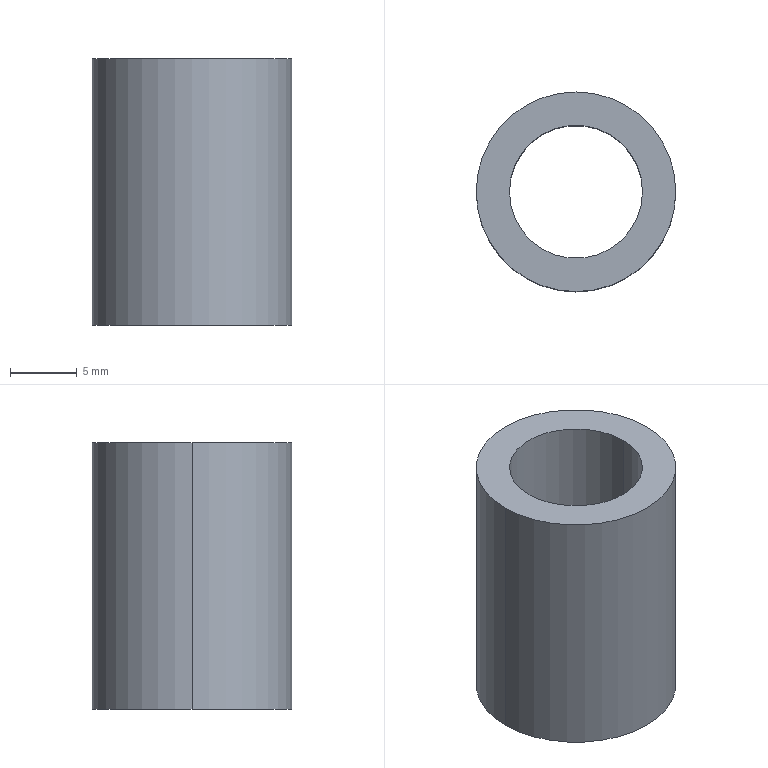Part | SolidWorks | features Extrusion 1 | 1 solid | 6 faces | box 15 x 15 x 20 mm | volume 1963 mm3 | cylinder 4 | plane 2 | commonest cylinder face diameters 10 x2 15 x2
STEP:
#1=CARTESIAN_POINT('',(-5.,0.,10.));
#2=VERTEX_POINT('',#1);
#3=CARTESIAN_POINT('',(5.,0.,10.));
#4=VERTEX_POINT('',#3);
#5=CARTESIAN_POINT('',(0.,0.,10.));
#6=DIRECTION('',(0.,0.,1.));
#7=DIRECTION('',(1.,0.,0.));
#8=AXIS2_PLACEMENT_3D('',#5,#6,#7);
#9=CIRCLE('',#8,5.);
#10=EDGE_CURVE('',#2,#4,#9,.T.);
#11=ORIENTED_EDGE('',*,*,#10,.T.);
#12=CARTESIAN_POINT('',(5.,0.,-10.));
#13=VERTEX_POINT('',#12);
#14=CARTESIAN_POINT('',(5.,0.,10.));
#15=DIRECTION('',(0.,0.,-1.));
#16=VECTOR('',#15,1000.);
#17=LINE('',#14,#16);
#18=EDGE_CURVE('',#4,#13,#17,.T.);
#19=ORIENTED_EDGE('',*,*,#18,.T.);
#20=CARTESIAN_POINT('',(-5.,0.,-10.));
#21=VERTEX_POINT('',#20);
#22=CARTESIAN_POINT('',(0.,0.,-10.));
#23=DIRECTION('',(0.,0.,1.));
#24=DIRECTION('',(1.,0.,0.));
#25=AXIS2_PLACEMENT_3D('',#22,#23,#24);
#26=CIRCLE('',#25,5.);
#27=EDGE_CURVE('',#21,#13,#26,.T.);
#28=ORIENTED_EDGE('',*,*,#27,.F.);
#29=CARTESIAN_POINT('',(-5.,0.,10.));
#30=DIRECTION('',(0.,0.,-1.));
#31=VECTOR('',#30,1000.);
#32=LINE('',#29,#31);
#33=EDGE_CURVE('',#2,#21,#32,.T.);
#34=ORIENTED_EDGE('',*,*,#33,.F.);
#35=EDGE_LOOP('',(#11,#19,#28,#34));
#36=FACE_OUTER_BOUND('',#35,.T.);
#37=CARTESIAN_POINT('',(0.,0.,10.));
#38=DIRECTION('',(0.,0.,-1.));
#39=DIRECTION('',(-1.,0.,0.));
#40=AXIS2_PLACEMENT_3D('',#37,#38,#39);
#41=CYLINDRICAL_SURFACE('',#40,5.);
#42=ADVANCED_FACE('',(#36),#41,.F.);
#43=CARTESIAN_POINT('',(7.5,0.,10.));
#44=VERTEX_POINT('',#43);
#45=CARTESIAN_POINT('',(-7.5,0.,10.));
#46=VERTEX_POINT('',#45);
#47=CARTESIAN_POINT('',(0.,0.,10.));
#48=DIRECTION('',(0.,0.,1.));
#49=DIRECTION('',(1.,0.,0.));
#50=AXIS2_PLACEMENT_3D('',#47,#48,#49);
#51=CIRCLE('',#50,7.5);
#52=EDGE_CURVE('',#44,#46,#51,.T.);
#53=ORIENTED_EDGE('',*,*,#52,.F.);
#54=CARTESIAN_POINT('',(7.5,0.,-10.));
#55=VERTEX_POINT('',#54);
#56=CARTESIAN_POINT('',(7.5,0.,10.));
#57=DIRECTION('',(0.,0.,-1.));
#58=VECTOR('',#57,1000.);
#59=LINE('',#56,#58);
#60=EDGE_CURVE('',#44,#55,#59,.T.);
#61=ORIENTED_EDGE('',*,*,#60,.T.);
#62=CARTESIAN_POINT('',(-7.5,0.,-10.));
#63=VERTEX_POINT('',#62);
#64=CARTESIAN_POINT('',(0.,0.,-10.));
#65=DIRECTION('',(0.,0.,1.));
#66=DIRECTION('',(1.,0.,0.));
#67=AXIS2_PLACEMENT_3D('',#64,#65,#66);
#68=CIRCLE('',#67,7.5);
#69=EDGE_CURVE('',#55,#63,#68,.T.);
#70=ORIENTED_EDGE('',*,*,#69,.T.);
#71=CARTESIAN_POINT('',(-7.5,0.,10.));
#72=DIRECTION('',(0.,0.,-1.));
#73=VECTOR('',#72,1000.);
#74=LINE('',#71,#73);
#75=EDGE_CURVE('',#46,#63,#74,.T.);
#76=ORIENTED_EDGE('',*,*,#75,.F.);
#77=EDGE_LOOP('',(#53,#61,#70,#76));
#78=FACE_OUTER_BOUND('',#77,.T.);
#79=CARTESIAN_POINT('',(0.,0.,10.));
#80=DIRECTION('',(0.,0.,-1.));
#81=DIRECTION('',(-1.,0.,0.));
#82=AXIS2_PLACEMENT_3D('',#79,#80,#81);
#83=CYLINDRICAL_SURFACE('',#82,7.5);
#84=ADVANCED_FACE('',(#78),#83,.T.);
#85=CARTESIAN_POINT('',(0.,0.,10.));
#86=DIRECTION('',(0.,0.,1.));
#87=DIRECTION('',(1.,0.,0.));
#88=AXIS2_PLACEMENT_3D('',#85,#86,#87);
#89=CIRCLE('',#88,7.5);
#90=EDGE_CURVE('',#46,#44,#89,.T.);
#91=ORIENTED_EDGE('',*,*,#90,.T.);
#92=ORIENTED_EDGE('',*,*,#52,.T.);
#93=EDGE_LOOP('',(#91,#92));
#94=FACE_OUTER_BOUND('',#93,.T.);
#95=ORIENTED_EDGE('',*,*,#10,.F.);
#96=CARTESIAN_POINT('',(0.,0.,10.));
#97=DIRECTION('',(0.,0.,1.));
#98=DIRECTION('',(1.,0.,0.));
#99=AXIS2_PLACEMENT_3D('',#96,#97,#98);
#100=CIRCLE('',#99,5.);
#101=EDGE_CURVE('',#4,#2,#100,.T.);
#102=ORIENTED_EDGE('',*,*,#101,.F.);
#103=EDGE_LOOP('',(#95,#102));
#104=FACE_BOUND('',#103,.T.);
#105=CARTESIAN_POINT('',(0.,0.,10.));
#106=DIRECTION('',(0.,0.,1.));
#107=DIRECTION('',(1.,0.,0.));
#108=AXIS2_PLACEMENT_3D('',#105,#106,#107);
#109=PLANE('',#108);
#110=ADVANCED_FACE('',(#94,#104),#109,.T.);
#111=CARTESIAN_POINT('',(0.,0.,-10.));
#112=DIRECTION('',(0.,0.,1.));
#113=DIRECTION('',(1.,0.,0.));
#114=AXIS2_PLACEMENT_3D('',#111,#112,#113);
#115=CIRCLE('',#114,7.5);
#116=EDGE_CURVE('',#63,#55,#115,.T.);
#117=ORIENTED_EDGE('',*,*,#116,.F.);
#118=ORIENTED_EDGE('',*,*,#69,.F.);
#119=EDGE_LOOP('',(#117,#118));
#120=FACE_OUTER_BOUND('',#119,.T.);
#121=ORIENTED_EDGE('',*,*,#27,.T.);
#122=CARTESIAN_POINT('',(0.,0.,-10.));
#123=DIRECTION('',(0.,0.,1.));
#124=DIRECTION('',(1.,0.,0.));
#125=AXIS2_PLACEMENT_3D('',#122,#123,#124);
#126=CIRCLE('',#125,5.);
#127=EDGE_CURVE('',#13,#21,#126,.T.);
#128=ORIENTED_EDGE('',*,*,#127,.T.);
#129=EDGE_LOOP('',(#121,#128));
#130=FACE_BOUND('',#129,.T.);
#131=CARTESIAN_POINT('',(0.,0.,-10.));
#132=DIRECTION('',(0.,0.,1.));
#133=DIRECTION('',(1.,0.,0.));
#134=AXIS2_PLACEMENT_3D('',#131,#132,#133);
#135=PLANE('',#134);
#136=ADVANCED_FACE('',(#120,#130),#135,.F.);
#137=ORIENTED_EDGE('',*,*,#60,.F.);
#138=ORIENTED_EDGE('',*,*,#90,.F.);
#139=ORIENTED_EDGE('',*,*,#75,.T.);
#140=ORIENTED_EDGE('',*,*,#116,.T.);
#141=EDGE_LOOP('',(#137,#138,#139,#140));
#142=FACE_OUTER_BOUND('',#141,.T.);
#143=CARTESIAN_POINT('',(0.,0.,10.));
#144=DIRECTION('',(0.,0.,-1.));
#145=DIRECTION('',(-1.,0.,0.));
#146=AXIS2_PLACEMENT_3D('',#143,#144,#145);
#147=CYLINDRICAL_SURFACE('',#146,7.5);
#148=ADVANCED_FACE('',(#142),#147,.T.);
#149=ORIENTED_EDGE('',*,*,#18,.F.);
#150=ORIENTED_EDGE('',*,*,#101,.T.);
#151=ORIENTED_EDGE('',*,*,#33,.T.);
#152=ORIENTED_EDGE('',*,*,#127,.F.);
#153=EDGE_LOOP('',(#149,#150,#151,#152));
#154=FACE_OUTER_BOUND('',#153,.T.);
#155=CARTESIAN_POINT('',(0.,0.,10.));
#156=DIRECTION('',(0.,0.,-1.));
#157=DIRECTION('',(-1.,0.,0.));
#158=AXIS2_PLACEMENT_3D('',#155,#156,#157);
#159=CYLINDRICAL_SURFACE('',#158,5.);
#160=ADVANCED_FACE('',(#154),#159,.F.);
#161=CLOSED_SHELL('',(#42,#84,#110,#136,#148,#160));
#162=MANIFOLD_SOLID_BREP('',#161);
#163=CARTESIAN_POINT('',(0.,0.,0.));
#164=DIRECTION('',(0.,0.,1.));
#165=DIRECTION('',(1.,0.,0.));
#166=AXIS2_PLACEMENT_3D('',#163,#164,#165);
#167=(LENGTH_UNIT()NAMED_UNIT(*)SI_UNIT(.MILLI.,.METRE.));
#168=UNCERTAINTY_MEASURE_WITH_UNIT(LENGTH_MEASURE(0.00001),#167,'','');
#169=(NAMED_UNIT(*)PLANE_ANGLE_UNIT()SI_UNIT($,.RADIAN.));
#170=(NAMED_UNIT(*)SI_UNIT($,.STERADIAN.)SOLID_ANGLE_UNIT());
#171=(GEOMETRIC_REPRESENTATION_CONTEXT(3)GLOBAL_UNCERTAINTY_ASSIGNED_CONTEXT((#168))GLOBAL_UNIT_ASSIGNED_CONTEXT((#167,#169,#170))REPRESENTATION_CONTEXT('',''));
#172=ADVANCED_BREP_SHAPE_REPRESENTATION('',(#162,#166),#171);